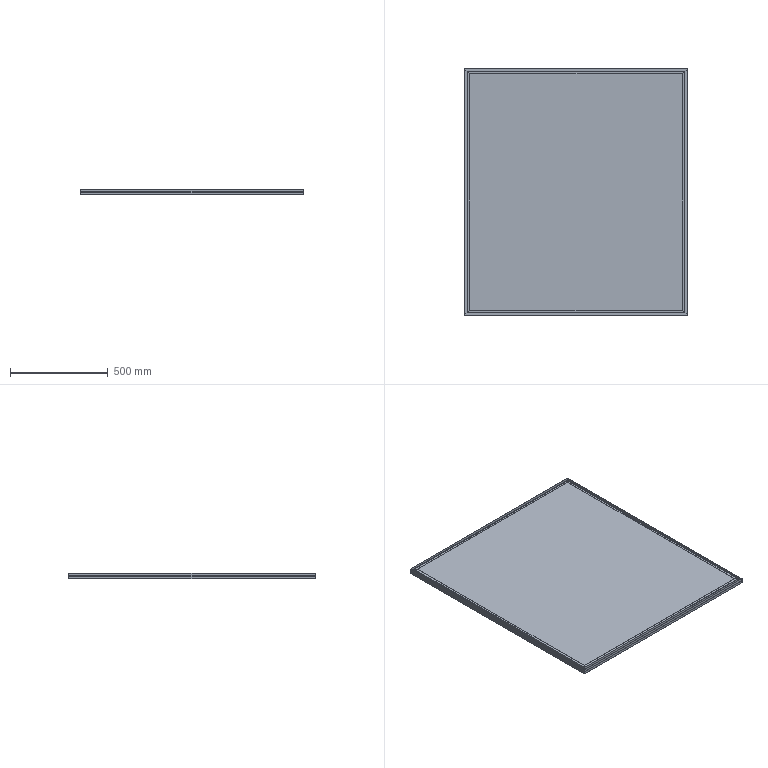Part | SolidWorks | features ICE 1, WeldMemberFeat 1, WeldmentFeature 1 | 5 solids | 78 faces | box 1140 x 1260 x 27 mm | volume 30852596 mm3 | plane 78